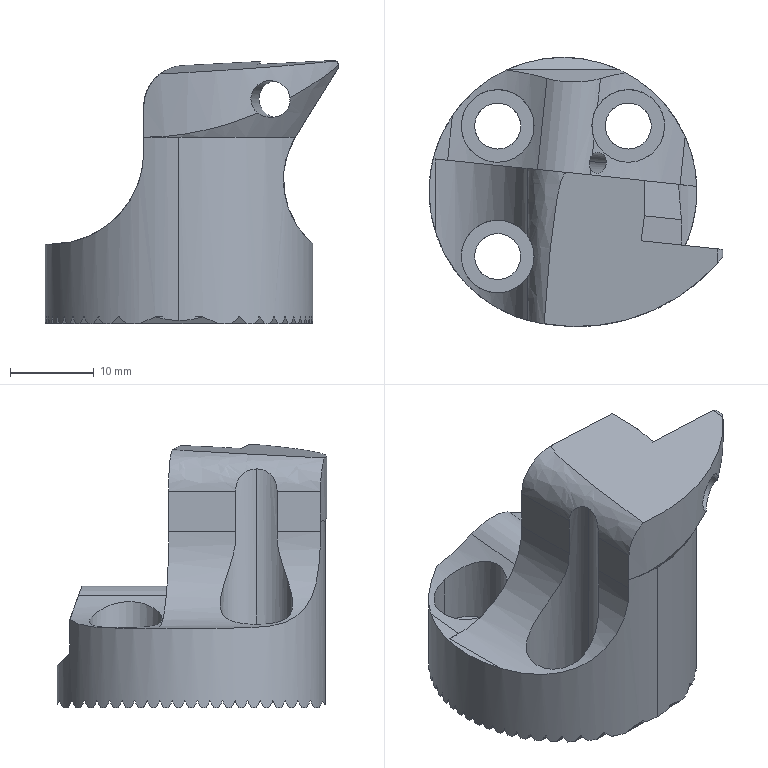NC program | Mastercam | posted with a generic post
Lines 4934 to 6578 of 7170:
(4 FEMR |TOOL - 5|DIA. OFF. - 5|LEN. - 5|TOOL DIA. - 4.)
N9924 T5 M6
N9926 G0 G54 G90 X45.762 Y19.276 C6. B-90. S4000 M3
N9928 G43 H5 Z52.023
N9930 Z3.023
N9932 G1 Z1.825 F2000.
N9934 G41 D5 X44.822 Y18.934 F600.
N9936 X30.436 Y13.698
N9938 X27.418 Y11.34
N9940 X31.243 Y11.54
N9942 X45.536 Y17.027
N9944 G40 X46.469 Y17.385
N9946 X45.078 Y21.156
N9948 G41 D5 X44.138 Y20.814
N9950 X29.455 Y15.469
N9952 X21.188 Y9.01
N9954 X31.664 Y9.56
N9956 X46.252 Y15.159
N9958 G40 X47.186 Y15.518
N9960 X45.762 Y19.276
N9962 Z1.627 F2000.
N9964 G41 D5 X44.822 Y18.934 F600.
N9966 X30.436 Y13.698
N9968 X27.418 Y11.34
N9970 X31.243 Y11.54
N9972 X45.536 Y17.027
N9974 G40 X46.469 Y17.385
N9976 X45.078 Y21.156
N9978 G41 D5 X44.138 Y20.814
N9980 X29.455 Y15.469
N9982 X21.188 Y9.01
N9984 X31.664 Y9.56
N9986 X46.252 Y15.159
N9988 G40 X47.186 Y15.518
N9990 X45.762 Y19.276
N9992 Z1.43 F2000.
N9994 G41 D5 X44.822 Y18.934 F600.
N9996 X30.436 Y13.698
N9998 X27.418 Y11.34
N100 X31.243 Y11.54
N102 X45.536 Y17.027
N104 G40 X46.469 Y17.385
N106 X45.078 Y21.156
N108 G41 D5 X44.138 Y20.814
N110 X29.455 Y15.469
N112 X21.188 Y9.01
N114 X31.664 Y9.56
N116 X46.252 Y15.159
N118 G40 X47.186 Y15.518
N120 X45.762 Y19.276
N122 Z1.232 F2000.
N124 G41 D5 X44.822 Y18.934 F600.
N126 X30.436 Y13.698
N128 X27.418 Y11.34
N130 X31.243 Y11.54
N132 X45.536 Y17.027
N134 G40 X46.469 Y17.385
N136 X45.078 Y21.156
N138 G41 D5 X44.138 Y20.814
N140 X29.455 Y15.469
N142 X21.188 Y9.01
N144 X31.664 Y9.56
N146 X46.252 Y15.159
N148 G40 X47.186 Y15.518
N150 X45.762 Y19.276
N152 Z1.035 F2000.
N154 G41 D5 X44.822 Y18.934 F600.
N156 X30.436 Y13.698
N158 X27.418 Y11.34
N160 X31.243 Y11.54
N162 X45.536 Y17.027
N164 G40 X46.469 Y17.385
N166 X45.078 Y21.156
N168 G41 D5 X44.138 Y20.814
N170 X29.455 Y15.469
N172 X21.188 Y9.01
N174 X31.664 Y9.56
N176 X46.252 Y15.159
N178 G40 X47.186 Y15.518
N180 X45.762 Y19.276
N182 Z.837 F2000.
N184 G41 D5 X44.822 Y18.934 F600.
N186 X30.436 Y13.698
N188 X27.418 Y11.34
N190 X31.243 Y11.54
N192 X45.536 Y17.027
N194 G40 X46.469 Y17.385
N196 X45.078 Y21.156
N198 G41 D5 X44.138 Y20.814
N200 X29.455 Y15.469
N202 X21.188 Y9.01
N204 X31.664 Y9.56
N206 X46.252 Y15.159
N208 G40 X47.186 Y15.518
N210 X45.762 Y19.276
N212 Z.64 F2000.
N214 G41 D5 X44.822 Y18.934 F600.
N216 X30.436 Y13.698
N218 X27.418 Y11.34
N220 X31.243 Y11.54
N222 X45.536 Y17.027
N224 G40 X46.469 Y17.385
N226 X45.078 Y21.156
N228 G41 D5 X44.138 Y20.814
N230 X29.455 Y15.469
N232 X21.188 Y9.01
N234 X31.664 Y9.56
N236 X46.252 Y15.159
N238 G40 X47.186 Y15.518
N240 X45.762 Y19.276
N242 Z.442 F2000.
N244 G41 D5 X44.822 Y18.934 F600.
N246 X30.436 Y13.698
N248 X27.418 Y11.34
N250 X31.243 Y11.54
N252 X45.536 Y17.027
N254 G40 X46.469 Y17.385
N256 X45.078 Y21.156
N258 G41 D5 X44.138 Y20.814
N260 X29.455 Y15.469
N262 X21.188 Y9.01
N264 X31.664 Y9.56
N266 X46.252 Y15.159
N268 G40 X47.186 Y15.518
N270 X45.762 Y19.276
N272 Z.245 F2000.
N274 G41 D5 X44.822 Y18.934 F600.
N276 X30.436 Y13.698
N278 X27.418 Y11.34
N280 X31.243 Y11.54
N282 X45.536 Y17.027
N284 G40 X46.469 Y17.385
N286 X45.078 Y21.156
N288 G41 D5 X44.138 Y20.814
N290 X29.455 Y15.469
N292 X21.188 Y9.01
N294 X31.664 Y9.56
N296 X46.252 Y15.159
N298 G40 X47.186 Y15.518
N300 X45.762 Y19.276
N302 Z.047 F2000.
N304 G41 D5 X44.822 Y18.934 F600.
N306 X30.436 Y13.698
N308 X27.418 Y11.34
N310 X31.243 Y11.54
N312 X45.536 Y17.027
N314 G40 X46.469 Y17.385
N316 X45.078 Y21.156
N318 G41 D5 X44.138 Y20.814
N320 X29.455 Y15.469
N322 X21.188 Y9.01
N324 X31.664 Y9.56
N326 X46.252 Y15.159
N328 G40 X47.186 Y15.518
N330 X45.762 Y19.276
N332 Z-.151 F2000.
N334 G41 D5 X44.822 Y18.934 F600.
N336 X30.436 Y13.698
N338 X27.418 Y11.34
N340 X31.243 Y11.54
N342 X45.536 Y17.027
N344 G40 X46.469 Y17.385
N346 X45.078 Y21.156
N348 G41 D5 X44.138 Y20.814
N350 X29.455 Y15.469
N352 X21.188 Y9.01
N354 X31.664 Y9.56
N356 X46.252 Y15.159
N358 G40 X47.186 Y15.518
N360 X45.762 Y19.276
N362 Z-.348 F2000.
N364 G41 D5 X44.822 Y18.934 F600.
N366 X30.436 Y13.698
N368 X27.418 Y11.34
N370 X31.243 Y11.54
N372 X45.536 Y17.027
N374 G40 X46.469 Y17.385
N376 X45.078 Y21.156
N378 G41 D5 X44.138 Y20.814
N380 X29.455 Y15.469
N382 X21.188 Y9.01
N384 X31.664 Y9.56
N386 X46.252 Y15.159
N388 G40 X47.186 Y15.518
N390 X45.762 Y19.276
N392 Z-.546 F2000.
N394 G41 D5 X44.822 Y18.934 F600.
N396 X30.436 Y13.698
N398 X27.418 Y11.34
N400 X31.243 Y11.54
N402 X45.536 Y17.027
N404 G40 X46.469 Y17.385
N406 X45.078 Y21.156
N408 G41 D5 X44.138 Y20.814
N410 X29.455 Y15.469
N412 X21.188 Y9.01
N414 X31.664 Y9.56
N416 X46.252 Y15.159
N418 G40 X47.186 Y15.518
N420 X45.762 Y19.276
N422 Z-.743 F2000.
N424 G41 D5 X44.822 Y18.934 F600.
N426 X30.436 Y13.698
N428 X27.418 Y11.34
N430 X31.243 Y11.54
N432 X45.536 Y17.027
N434 G40 X46.469 Y17.385
N436 X45.078 Y21.156
N438 G41 D5 X44.138 Y20.814
N440 X29.455 Y15.469
N442 X21.188 Y9.01
N444 X31.664 Y9.56
N446 X46.252 Y15.159
N448 G40 X47.186 Y15.518
N450 X45.762 Y19.276
N452 Z-.941 F2000.
N454 G41 D5 X44.822 Y18.934 F600.
N456 X30.436 Y13.698
N458 X27.418 Y11.34
N460 X31.243 Y11.54
N462 X45.536 Y17.027
N464 G40 X46.469 Y17.385
N466 X45.078 Y21.156
N468 G41 D5 X44.138 Y20.814
N470 X29.455 Y15.469
N472 X21.188 Y9.01
N474 X31.664 Y9.56
N476 X46.252 Y15.159
N478 G40 X47.186 Y15.518
N480 X45.762 Y19.276
N482 Z-1.138 F2000.
N484 G41 D5 X44.822 Y18.934 F600.
N486 X30.436 Y13.698
N488 X27.418 Y11.34
N490 X31.243 Y11.54
N492 X45.536 Y17.027
N494 G40 X46.469 Y17.385
N496 X45.078 Y21.156
N498 G41 D5 X44.138 Y20.814
N500 X29.455 Y15.469
N502 X21.188 Y9.01
N504 X31.664 Y9.56
N506 X46.252 Y15.159
N508 G40 X47.186 Y15.518
N510 X45.762 Y19.276
N512 Z-1.336 F2000.
N514 G41 D5 X44.822 Y18.934 F600.
N516 X30.436 Y13.698
N518 X27.418 Y11.34
N520 X31.243 Y11.54
N522 X45.536 Y17.027
N524 G40 X46.469 Y17.385
N526 X45.078 Y21.156
N528 G41 D5 X44.138 Y20.814
N530 X29.455 Y15.469
N532 X21.188 Y9.01
N534 X31.664 Y9.56
N536 X46.252 Y15.159
N538 G40 X47.186 Y15.518
N540 X45.762 Y19.276
N542 Z-1.534 F2000.
N544 G41 D5 X44.822 Y18.934 F600.
N546 X30.436 Y13.698
N548 X27.418 Y11.34
N550 X31.243 Y11.54
N552 X45.536 Y17.027
N554 G40 X46.469 Y17.385
N556 X45.078 Y21.156
N558 G41 D5 X44.138 Y20.814
N560 X29.455 Y15.469
N562 X21.188 Y9.01
N564 X31.664 Y9.56
N566 X46.252 Y15.159
N568 G40 X47.186 Y15.518
N570 X45.762 Y19.276
N572 Z-1.731 F2000.
N574 G41 D5 X44.822 Y18.934 F600.
N576 X30.436 Y13.698
N578 X27.418 Y11.34
N580 X31.243 Y11.54
N582 X45.536 Y17.027
N584 G40 X46.469 Y17.385
N586 X45.078 Y21.156
N588 G41 D5 X44.138 Y20.814
N590 X29.455 Y15.469
N592 X21.188 Y9.01
N594 X31.664 Y9.56
N596 X46.252 Y15.159
N598 G40 X47.186 Y15.518
N600 X45.762 Y19.276
N602 Z-1.929 F2000.
N604 G41 D5 X44.822 Y18.934 F600.
N606 X30.436 Y13.698
N608 X27.418 Y11.34
N610 X31.243 Y11.54
N612 X45.536 Y17.027
N614 G40 X46.469 Y17.385
N616 X45.078 Y21.156
N618 G41 D5 X44.138 Y20.814
N620 X29.455 Y15.469
N622 X21.188 Y9.01
N624 X31.664 Y9.56
N626 X46.252 Y15.159
N628 G40 X47.186 Y15.518
N630 X45.762 Y19.276
N632 Z-2.126 F2000.
N634 G41 D5 X44.822 Y18.934 F600.
N636 X30.436 Y13.698
N638 X27.418 Y11.34
N640 X31.243 Y11.54
N642 X45.536 Y17.027
N644 G40 X46.469 Y17.385
N646 X45.078 Y21.156
N648 G41 D5 X44.138 Y20.814
N650 X29.455 Y15.469
N652 X21.188 Y9.01
N654 X31.664 Y9.56
N656 X46.252 Y15.159
N658 G40 X47.186 Y15.518
N660 X45.762 Y19.276
N662 Z-2.324 F2000.
N664 G41 D5 X44.822 Y18.934 F600.
N666 X30.436 Y13.698
N668 X27.418 Y11.34
N670 X31.243 Y11.54
N672 X45.536 Y17.027
N674 G40 X46.469 Y17.385
N676 X45.078 Y21.156
N678 G41 D5 X44.138 Y20.814
N680 X29.455 Y15.469
N682 X21.188 Y9.01
N684 X31.664 Y9.56
N686 X46.252 Y15.159
N688 G40 X47.186 Y15.518
N690 X45.762 Y19.276
N692 Z-2.521 F2000.
N694 G41 D5 X44.822 Y18.934 F600.
N696 X30.436 Y13.698
N698 X27.418 Y11.34
N700 X31.243 Y11.54
N702 X45.536 Y17.027
N704 G40 X46.469 Y17.385
N706 X45.078 Y21.156
N708 G41 D5 X44.138 Y20.814
N710 X29.455 Y15.469
N712 X21.188 Y9.01
N714 X31.664 Y9.56
N716 X46.252 Y15.159
N718 G40 X47.186 Y15.518
N720 X45.762 Y19.276
N722 Z-2.719 F2000.
N724 G41 D5 X44.822 Y18.934 F600.
N726 X30.436 Y13.698
N728 X27.418 Y11.34
N730 X31.243 Y11.54
N732 X45.536 Y17.027
N734 G40 X46.469 Y17.385
N736 X45.078 Y21.156
N738 G41 D5 X44.138 Y20.814
N740 X29.455 Y15.469
N742 X21.188 Y9.01
N744 X31.664 Y9.56
N746 X46.252 Y15.159
N748 G40 X47.186 Y15.518
N750 X45.762 Y19.276
N752 Z-2.916 F2000.
N754 G41 D5 X44.822 Y18.934 F600.
N756 X30.436 Y13.698
N758 X27.418 Y11.34
N760 X31.243 Y11.54
N762 X45.536 Y17.027
N764 G40 X46.469 Y17.385
N766 X45.078 Y21.156
N768 G41 D5 X44.138 Y20.814
N770 X29.455 Y15.469
N772 X21.188 Y9.01
N774 X31.664 Y9.56
N776 X46.252 Y15.159
N778 G40 X47.186 Y15.518
N780 X45.762 Y19.276
N782 Z-3.114 F2000.
N784 G41 D5 X44.822 Y18.934 F600.
N786 X30.436 Y13.698
N788 X27.418 Y11.34
N790 X31.243 Y11.54
N792 X45.536 Y17.027
N794 G40 X46.469 Y17.385
N796 X45.078 Y21.156
N798 G41 D5 X44.138 Y20.814
N800 X29.455 Y15.469
N802 X21.188 Y9.01
N804 X31.664 Y9.56
N806 X46.252 Y15.159
N808 G40 X47.186 Y15.518
N810 X45.762 Y19.276
N812 Z-3.312 F2000.
N814 G41 D5 X44.822 Y18.934 F600.
N816 X30.436 Y13.698
N818 X27.418 Y11.34
N820 X31.243 Y11.54
N822 X45.536 Y17.027
N824 G40 X46.469 Y17.385
N826 X45.078 Y21.156
N828 G41 D5 X44.138 Y20.814
N830 X29.455 Y15.469
N832 X21.188 Y9.01
N834 X31.664 Y9.56
N836 X46.252 Y15.159
N838 G40 X47.186 Y15.518
N840 X45.762 Y19.276
N842 Z-3.509 F2000.
N844 G41 D5 X44.822 Y18.934 F600.
N846 X30.436 Y13.698
N848 X27.418 Y11.34
N850 X31.243 Y11.54
N852 X45.536 Y17.027
N854 G40 X46.469 Y17.385
N856 X45.078 Y21.156
N858 G41 D5 X44.138 Y20.814
N860 X29.455 Y15.469
N862 X21.188 Y9.01
N864 X31.664 Y9.56
N866 X46.252 Y15.159
N868 G40 X47.186 Y15.518
N870 X45.762 Y19.276
N872 Z-3.707 F2000.
N874 G41 D5 X44.822 Y18.934 F600.
N876 X30.436 Y13.698
N878 X27.418 Y11.34
N880 X31.243 Y11.54
N882 X45.536 Y17.027
N884 G40 X46.469 Y17.385
N886 X45.078 Y21.156
N888 G41 D5 X44.138 Y20.814
N890 X29.455 Y15.469
N892 X21.188 Y9.01
N894 X31.664 Y9.56
N896 X46.252 Y15.159
N898 G40 X47.186 Y15.518
N900 X45.762 Y19.276
N902 Z-3.904 F2000.
N904 G41 D5 X44.822 Y18.934 F600.
N906 X30.436 Y13.698
N908 X27.418 Y11.34
N910 X31.243 Y11.54
N912 X45.536 Y17.027
N914 G40 X46.469 Y17.385
N916 X45.078 Y21.156
N918 G41 D5 X44.138 Y20.814
N920 X29.455 Y15.469
N922 X21.188 Y9.01
N924 X31.664 Y9.56
N926 X46.252 Y15.159
N928 G40 X47.186 Y15.518
N930 X45.762 Y19.276
N932 Z-4.102 F2000.
N934 G41 D5 X44.822 Y18.934 F600.
N936 X30.436 Y13.698
N938 X27.418 Y11.34
N940 X31.243 Y11.54
N942 X45.536 Y17.027
N944 G40 X46.469 Y17.385
N946 X45.078 Y21.156
N948 G41 D5 X44.138 Y20.814
N950 X29.455 Y15.469
N952 X21.188 Y9.01
N954 X31.664 Y9.56
N956 X46.252 Y15.159
N958 G40 X47.186 Y15.518
N960 X45.762 Y19.276
N962 Z-4.299 F2000.
N964 G41 D5 X44.822 Y18.934 F600.
N966 X30.436 Y13.698
N968 X27.418 Y11.34
N970 X31.243 Y11.54
N972 X45.536 Y17.027
N974 G40 X46.469 Y17.385
N976 X45.078 Y21.156
N978 G41 D5 X44.138 Y20.814
N980 X29.455 Y15.469
N982 X21.188 Y9.01
N984 X31.664 Y9.56
N986 X46.252 Y15.159
N988 G40 X47.186 Y15.518
N990 X45.762 Y19.276
N992 Z-4.497 F2000.
N994 G41 D5 X44.822 Y18.934 F600.
N996 X30.436 Y13.698
N998 X27.418 Y11.34
N1000 X31.243 Y11.54
N1002 X45.536 Y17.027
N1004 G40 X46.469 Y17.385
N1006 X45.078 Y21.156
N1008 G41 D5 X44.138 Y20.814
N1010 X29.455 Y15.469
N1012 X21.188 Y9.01
N1014 X31.664 Y9.56
N1016 X46.252 Y15.159
N1018 G40 X47.186 Y15.518
N1020 X45.762 Y19.276
N1022 Z-4.694 F2000.
N1024 G41 D5 X44.822 Y18.934 F600.
N1026 X30.436 Y13.698
N1028 X27.418 Y11.34
N1030 X31.243 Y11.54
N1032 X45.536 Y17.027
N1034 G40 X46.469 Y17.385
N1036 X45.078 Y21.156
N1038 G41 D5 X44.138 Y20.814
N1040 X29.455 Y15.469
N1042 X21.188 Y9.01
N1044 X31.664 Y9.56
N1046 X46.252 Y15.159
N1048 G40 X47.186 Y15.518
N1050 X45.762 Y19.276
N1052 Z-4.892 F2000.
N1054 G41 D5 X44.822 Y18.934 F600.
N1056 X30.436 Y13.698
N1058 X27.418 Y11.34
N1060 X31.243 Y11.54
N1062 X45.536 Y17.027
N1064 G40 X46.469 Y17.385
N1066 X45.078 Y21.156
N1068 G41 D5 X44.138 Y20.814
N1070 X29.455 Y15.469
N1072 X21.188 Y9.01
N1074 X31.664 Y9.56
N1076 X46.252 Y15.159
N1078 G40 X47.186 Y15.518
N1080 X45.762 Y19.276
N1082 Z-5.09 F2000.
N1084 G41 D5 X44.822 Y18.934 F600.
N1086 X30.436 Y13.698
N1088 X27.418 Y11.34
N1090 X31.243 Y11.54
N1092 X45.536 Y17.027
N1094 G40 X46.469 Y17.385
N1096 X45.078 Y21.156
N1098 G41 D5 X44.138 Y20.814
N1100 X29.455 Y15.469
N1102 X21.188 Y9.01
N1104 X31.664 Y9.56
N1106 X46.252 Y15.159
N1108 G40 X47.186 Y15.518
N1110 X45.762 Y19.276
N1112 Z-5.287 F2000.
N1114 G41 D5 X44.822 Y18.934 F600.
N1116 X30.436 Y13.698
N1118 X27.418 Y11.34
N1120 X31.243 Y11.54
N1122 X45.536 Y17.027
N1124 G40 X46.469 Y17.385
N1126 X45.078 Y21.156
N1128 G41 D5 X44.138 Y20.814
N1130 X29.455 Y15.469
N1132 X21.188 Y9.01
N1134 X31.664 Y9.56
N1136 X46.252 Y15.159
N1138 G40 X47.186 Y15.518
N1140 X45.762 Y19.276
N1142 Z-5.485 F2000.
N1144 G41 D5 X44.822 Y18.934 F600.
N1146 X30.436 Y13.698
N1148 X27.418 Y11.34
N1150 X31.243 Y11.54
N1152 X45.536 Y17.027
N1154 G40 X46.469 Y17.385
N1156 X45.078 Y21.156
N1158 G41 D5 X44.138 Y20.814
N1160 X29.455 Y15.469
N1162 X21.188 Y9.01
N1164 X31.664 Y9.56
N1166 X46.252 Y15.159
N1168 G40 X47.186 Y15.518
N1170 X45.762 Y19.276
N1172 Z-5.682 F2000.
N1174 G41 D5 X44.822 Y18.934 F600.
N1176 X30.436 Y13.698
N1178 X27.418 Y11.34
N1180 X31.243 Y11.54
N1182 X45.536 Y17.027
N1184 G40 X46.469 Y17.385
N1186 X45.078 Y21.156
N1188 G41 D5 X44.138 Y20.814
N1190 X29.455 Y15.469
N1192 X21.188 Y9.01
N1194 X31.664 Y9.56
N1196 X46.252 Y15.159
N1198 G40 X47.186 Y15.518
N1200 X45.762 Y19.276
N1202 Z-5.88 F2000.
N1204 G41 D5 X44.822 Y18.934 F600.
N1206 X30.436 Y13.698
N1208 X27.418 Y11.34
N1210 X31.243 Y11.54
N1212 X45.536 Y17.027
N1214 G40 X46.469 Y17.385
N1216 X45.078 Y21.156
N1218 G41 D5 X44.138 Y20.814
N1220 X29.455 Y15.469
N1222 X21.188 Y9.01
N1224 X31.664 Y9.56
N1226 X46.252 Y15.159
N1228 G40 X47.186 Y15.518
N1230 X45.762 Y19.276
N1232 Z-6.077 F2000.
N1234 G41 D5 X44.822 Y18.934 F600.
N1236 X30.436 Y13.698
N1238 X27.418 Y11.34
N1240 X31.243 Y11.54
N1242 X45.536 Y17.027
N1244 G40 X46.469 Y17.385
N1246 X45.078 Y21.156
N1248 G41 D5 X44.138 Y20.814
N1250 X29.455 Y15.469
N1252 X21.188 Y9.01
N1254 X31.664 Y9.56
N1256 X46.252 Y15.159
N1258 G40 X47.186 Y15.518
N1260 G0 Z52.023
N1262 M5
N1264 G0 G28 G91 Z0.
N1266 G28 C0. B0.
N1268 M01
N1270 G0 G17 G40 G80 G90 G94 G98
N1272 G0 G28 G91 Z0.
(3 FEMR |TOOL - 6|DIA. OFF. - 6|LEN. - 6|TOOL DIA. - 3.)
N1274 T6 M6
N1276 G0 G54 G90 X22.325 Y9.265 C6. B-90. S4500 M3
N1278 G43 H6 Z51.993
N1280 Z2.993
N1282 G1 Z1.796 F2000.
N1284 G41 D6 X22.017 Y9.659 F400.
N1286 G3 X21.623 Y9.851 I-.394 J-.308
N1288 X21.316 Y9.745 J-.5
N1290 G1 X20.155 Y8.838
N1292 X14.158 Y6.596
N1294 G3 X14.027 Y6.408 I.07 J-.188
N1296 X14.228 Y6.207 I.201
N1298 X14.298 Y6.221 J.201
N1300 G1 X20.295 Y8.463
N1302 X21.785 Y8.541
N1304 G3 X22.259 Y9.04 I-.026 J.499
N1306 X22.258 Y9.067 I-.5
N1308 G1 G40 X22.232 Y9.566
N1310 X22.325 Y9.265
N1312 Z1.599 F2000.
N1314 G41 D6 X22.017 Y9.659 F400.
N1316 G3 X21.623 Y9.851 I-.394 J-.308
N1318 X21.316 Y9.745 J-.5
N1320 G1 X20.155 Y8.838
N1322 X14.158 Y6.596
N1324 G3 X14.027 Y6.408 I.07 J-.188
N1326 X14.228 Y6.207 I.201
N1328 X14.298 Y6.221 J.201
N1330 G1 X20.295 Y8.463
N1332 X21.785 Y8.541
N1334 G3 X22.259 Y9.04 I-.026 J.499
N1336 X22.258 Y9.067 I-.5
N1338 G1 G40 X22.232 Y9.566
N1340 X22.325 Y9.265
N1342 Z1.402 F2000.
N1344 G41 D6 X22.017 Y9.659 F400.
N1346 G3 X21.623 Y9.851 I-.394 J-.308
N1348 X21.316 Y9.745 J-.5
N1350 G1 X20.155 Y8.838
N1352 X14.158 Y6.596
N1354 G3 X14.027 Y6.408 I.07 J-.188
N1356 X14.228 Y6.207 I.201
N1358 X14.298 Y6.221 J.201
N1360 G1 X20.295 Y8.463
N1362 X21.785 Y8.541
N1364 G3 X22.259 Y9.04 I-.026 J.499
N1366 X22.258 Y9.067 I-.5
N1368 G1 G40 X22.232 Y9.566
N1370 X22.325 Y9.265
N1372 Z1.205 F2000.
N1374 G41 D6 X22.017 Y9.659 F400.
N1376 G3 X21.623 Y9.851 I-.394 J-.308
N1378 X21.316 Y9.745 J-.5
N1380 G1 X20.155 Y8.838
N1382 X14.158 Y6.596
N1384 G3 X14.027 Y6.408 I.07 J-.188
N1386 X14.228 Y6.207 I.201
N1388 X14.298 Y6.221 J.201
N1390 G1 X20.295 Y8.463
N1392 X21.785 Y8.541
N1394 G3 X22.259 Y9.04 I-.026 J.499
N1396 X22.258 Y9.067 I-.5
N1398 G1 G40 X22.232 Y9.566
N1400 X22.325 Y9.265
N1402 Z1.008 F2000.
N1404 G41 D6 X22.017 Y9.659 F400.
N1406 G3 X21.623 Y9.851 I-.394 J-.308
N1408 X21.316 Y9.745 J-.5
N1410 G1 X20.155 Y8.838
N1412 X14.158 Y6.596
N1414 G3 X14.027 Y6.408 I.07 J-.188
N1416 X14.228 Y6.207 I.201
N1418 X14.298 Y6.221 J.201
N1420 G1 X20.295 Y8.463
N1422 X21.785 Y8.541
N1424 G3 X22.259 Y9.04 I-.026 J.499
N1426 X22.258 Y9.067 I-.5
N1428 G1 G40 X22.232 Y9.566
N1430 X22.325 Y9.265
N1432 Z.812 F2000.
N1434 G41 D6 X22.017 Y9.659 F400.
N1436 G3 X21.623 Y9.851 I-.394 J-.308
N1438 X21.316 Y9.745 J-.5
N1440 G1 X20.155 Y8.838
N1442 X14.158 Y6.596
N1444 G3 X14.027 Y6.408 I.07 J-.188
N1446 X14.228 Y6.207 I.201
N1448 X14.298 Y6.221 J.201
N1450 G1 X20.295 Y8.463
N1452 X21.785 Y8.541
N1454 G3 X22.259 Y9.04 I-.026 J.499
N1456 X22.258 Y9.067 I-.5
N1458 G1 G40 X22.232 Y9.566
N1460 X22.325 Y9.265
N1462 Z.615 F2000.
N1464 G41 D6 X22.017 Y9.659 F400.
N1466 G3 X21.623 Y9.851 I-.394 J-.308
N1468 X21.316 Y9.745 J-.5
N1470 G1 X20.155 Y8.838
N1472 X14.158 Y6.596
N1474 G3 X14.027 Y6.408 I.07 J-.188
N1476 X14.228 Y6.207 I.201
N1478 X14.298 Y6.221 J.201
N1480 G1 X20.295 Y8.463
N1482 X21.785 Y8.541
N1484 G3 X22.259 Y9.04 I-.026 J.499
N1486 X22.258 Y9.067 I-.5
N1488 G1 G40 X22.232 Y9.566
N1490 X22.325 Y9.265
N1492 Z.418 F2000.
N1494 G41 D6 X22.017 Y9.659 F400.
N1496 G3 X21.623 Y9.851 I-.394 J-.308
N1498 X21.316 Y9.745 J-.5
N1500 G1 X20.155 Y8.838
N1502 X14.158 Y6.596
N1504 G3 X14.027 Y6.408 I.07 J-.188
N1506 X14.228 Y6.207 I.201
N1508 X14.298 Y6.221 J.201
N1510 G1 X20.295 Y8.463
N1512 X21.785 Y8.541
N1514 G3 X22.259 Y9.04 I-.026 J.499
N1516 X22.258 Y9.067 I-.5
N1518 G1 G40 X22.232 Y9.566
N1520 X22.325 Y9.265
N1522 Z.221 F2000.
N1524 G41 D6 X22.017 Y9.659 F400.
N1526 G3 X21.623 Y9.851 I-.394 J-.308
N1528 X21.316 Y9.745 J-.5
N1530 G1 X20.155 Y8.838
N1532 X14.158 Y6.596
N1534 G3 X14.027 Y6.408 I.07 J-.188
N1536 X14.228 Y6.207 I.201
N1538 X14.298 Y6.221 J.201
N1540 G1 X20.295 Y8.463
N1542 X21.785 Y8.541
N1544 G3 X22.259 Y9.04 I-.026 J.499
N1546 X22.258 Y9.067 I-.5
N1548 G1 G40 X22.232 Y9.566
N1550 X22.325 Y9.265
N1552 Z.024 F2000.
N1554 G41 D6 X22.017 Y9.659 F400.
N1556 G3 X21.623 Y9.851 I-.394 J-.308
N1558 X21.316 Y9.745 J-.5
N1560 G1 X20.155 Y8.838
N1562 X14.158 Y6.596
N1564 G3 X14.027 Y6.408 I.07 J-.188
N1566 X14.228 Y6.207 I.201
N1568 X14.298 Y6.221 J.201
N1570 G1 X20.295 Y8.463
N1572 X21.785 Y8.541
N1574 G3 X22.259 Y9.04 I-.026 J.499
N1576 X22.258 Y9.067 I-.5
N1578 G1 G40 X22.232 Y9.566
N1580 X22.325 Y9.265
N1582 Z-.173 F2000.
N1584 G41 D6 X22.017 Y9.659 F400.
N1586 G3 X21.623 Y9.851 I-.394 J-.308
N1588 X21.316 Y9.745 J-.5
N1590 G1 X20.155 Y8.838
N1592 X14.158 Y6.596
N1594 G3 X14.027 Y6.408 I.07 J-.188
N1596 X14.228 Y6.207 I.201
N1598 X14.298 Y6.221 J.201
N1600 G1 X20.295 Y8.463
N1602 X21.785 Y8.541
N1604 G3 X22.259 Y9.04 I-.026 J.499
N1606 X22.258 Y9.067 I-.5
N1608 G1 G40 X22.232 Y9.566
N1610 X22.325 Y9.265
N1612 Z-.369 F2000.
N1614 G41 D6 X22.017 Y9.659 F400.
N1616 G3 X21.623 Y9.851 I-.394 J-.308
N1618 X21.316 Y9.745 J-.5
N1620 G1 X20.155 Y8.838
N1622 X14.158 Y6.596
N1624 G3 X14.027 Y6.408 I.07 J-.188
N1626 X14.228 Y6.207 I.201
N1628 X14.298 Y6.221 J.201
N1630 G1 X20.295 Y8.463
N1632 X21.785 Y8.541
N1634 G3 X22.259 Y9.04 I-.026 J.499
N1636 X22.258 Y9.067 I-.5
N1638 G1 G40 X22.232 Y9.566
N1640 X22.325 Y9.265
N1642 Z-.566 F2000.
N1644 G41 D6 X22.017 Y9.659 F400.
N1646 G3 X21.623 Y9.851 I-.394 J-.308
N1648 X21.316 Y9.745 J-.5
N1650 G1 X20.155 Y8.838
N1652 X14.158 Y6.596
N1654 G3 X14.027 Y6.408 I.07 J-.188
N1656 X14.228 Y6.207 I.201
N1658 X14.298 Y6.221 J.201
N1660 G1 X20.295 Y8.463
N1662 X21.785 Y8.541
N1664 G3 X22.259 Y9.04 I-.026 J.499
N1666 X22.258 Y9.067 I-.5
N1668 G1 G40 X22.232 Y9.566
N1670 X22.325 Y9.265
N1672 Z-.763 F2000.
N1674 G41 D6 X22.017 Y9.659 F400.
N1676 G3 X21.623 Y9.851 I-.394 J-.308
N1678 X21.316 Y9.745 J-.5
N1680 G1 X20.155 Y8.838
N1682 X14.158 Y6.596
N1684 G3 X14.027 Y6.408 I.07 J-.188
N1686 X14.228 Y6.207 I.201
N1688 X14.298 Y6.221 J.201
N1690 G1 X20.295 Y8.463
N1692 X21.785 Y8.541
N1694 G3 X22.259 Y9.04 I-.026 J.499
N1696 X22.258 Y9.067 I-.5
N1698 G1 G40 X22.232 Y9.566
N1700 X22.325 Y9.265
N1702 Z-.96 F2000.
N1704 G41 D6 X22.017 Y9.659 F400.
N1706 G3 X21.623 Y9.851 I-.394 J-.308
N1708 X21.316 Y9.745 J-.5
N1710 G1 X20.155 Y8.838
N1712 X14.158 Y6.596
N1714 G3 X14.027 Y6.408 I.07 J-.188
N1716 X14.228 Y6.207 I.201
N1718 X14.298 Y6.221 J.201
N1720 G1 X20.295 Y8.463
N1722 X21.785 Y8.541
N1724 G3 X22.259 Y9.04 I-.026 J.499
N1726 X22.258 Y9.067 I-.5
N1728 G1 G40 X22.232 Y9.566
N1730 X22.325 Y9.265
N1732 Z-1.157 F2000.
N1734 G41 D6 X22.017 Y9.659 F400.
N1736 G3 X21.623 Y9.851 I-.394 J-.308
N1738 X21.316 Y9.745 J-.5
N1740 G1 X20.155 Y8.838
N1742 X14.158 Y6.596
N1744 G3 X14.027 Y6.408 I.07 J-.188
N1746 X14.228 Y6.207 I.201
N1748 X14.298 Y6.221 J.201
N1750 G1 X20.295 Y8.463
N1752 X21.785 Y8.541
N1754 G3 X22.259 Y9.04 I-.026 J.499
N1756 X22.258 Y9.067 I-.5
N1758 G1 G40 X22.232 Y9.566
N1760 X22.325 Y9.265
N1762 Z-1.354 F2000.
N1764 G41 D6 X22.017 Y9.659 F400.
N1766 G3 X21.623 Y9.851 I-.394 J-.308
N1768 X21.316 Y9.745 J-.5
N1770 G1 X20.155 Y8.838
N1772 X14.158 Y6.596
N1774 G3 X14.027 Y6.408 I.07 J-.188
N1776 X14.228 Y6.207 I.201
N1778 X14.298 Y6.221 J.201
N1780 G1 X20.295 Y8.463
N1782 X21.785 Y8.541
N1784 G3 X22.259 Y9.04 I-.026 J.499
N1786 X22.258 Y9.067 I-.5
N1788 G1 G40 X22.232 Y9.566
N1790 X22.325 Y9.265
N1792 Z-1.55 F2000.
N1794 G41 D6 X22.017 Y9.659 F400.
N1796 G3 X21.623 Y9.851 I-.394 J-.308
N1798 X21.316 Y9.745 J-.5
N1800 G1 X20.155 Y8.838
N1802 X14.158 Y6.596
N1804 G3 X14.027 Y6.408 I.07 J-.188
N1806 X14.228 Y6.207 I.201
N1808 X14.298 Y6.221 J.201
N1810 G1 X20.295 Y8.463
N1812 X21.785 Y8.541
N1814 G3 X22.259 Y9.04 I-.026 J.499
N1816 X22.258 Y9.067 I-.5
N1818 G1 G40 X22.232 Y9.566
N1820 X22.325 Y9.265
N1822 Z-1.747 F2000.
N1824 G41 D6 X22.017 Y9.659 F400.
N1826 G3 X21.623 Y9.851 I-.394 J-.308
N1828 X21.316 Y9.745 J-.5
N1830 G1 X20.155 Y8.838
N1832 X14.158 Y6.596
N1834 G3 X14.027 Y6.408 I.07 J-.188
N1836 X14.228 Y6.207 I.201
N1838 X14.298 Y6.221 J.201
N1840 G1 X20.295 Y8.463
N1842 X21.785 Y8.541
N1844 G3 X22.259 Y9.04 I-.026 J.499
N1846 X22.258 Y9.067 I-.5
N1848 G1 G40 X22.232 Y9.566
N1850 X22.325 Y9.265
N1852 Z-1.944 F2000.
N1854 G41 D6 X22.017 Y9.659 F400.
N1856 G3 X21.623 Y9.851 I-.394 J-.308
N1858 X21.316 Y9.745 J-.5
N1860 G1 X20.155 Y8.838
N1862 X14.158 Y6.596
N1864 G3 X14.027 Y6.408 I.07 J-.188
N1866 X14.228 Y6.207 I.201
N1868 X14.298 Y6.221 J.201
N1870 G1 X20.295 Y8.463
N1872 X21.785 Y8.541
N1874 G3 X22.259 Y9.04 I-.026 J.499
N1876 X22.258 Y9.067 I-.5
N1878 G1 G40 X22.232 Y9.566
N1880 X22.325 Y9.265
N1882 Z-2.141 F2000.
N1884 G41 D6 X22.017 Y9.659 F400.
N1886 G3 X21.623 Y9.851 I-.394 J-.308
N1888 X21.316 Y9.745 J-.5
N1890 G1 X20.155 Y8.838
N1892 X14.158 Y6.596
N1894 G3 X14.027 Y6.408 I.07 J-.188
N1896 X14.228 Y6.207 I.201
N1898 X14.298 Y6.221 J.201
N1900 G1 X20.295 Y8.463
N1902 X21.785 Y8.541
N1904 G3 X22.259 Y9.04 I-.026 J.499
N1906 X22.258 Y9.067 I-.5
N1908 G1 G40 X22.232 Y9.566
N1910 X22.325 Y9.265
N1912 Z-2.338 F2000.
N1914 G41 D6 X22.017 Y9.659 F400.
N1916 G3 X21.623 Y9.851 I-.394 J-.308
N1918 X21.316 Y9.745 J-.5
N1920 G1 X20.155 Y8.838
N1922 X14.158 Y6.596
N1924 G3 X14.027 Y6.408 I.07 J-.188
N1926 X14.228 Y6.207 I.201
N1928 X14.298 Y6.221 J.201
N1930 G1 X20.295 Y8.463
N1932 X21.785 Y8.541
N1934 G3 X22.259 Y9.04 I-.026 J.499
N1936 X22.258 Y9.067 I-.5
N1938 G1 G40 X22.232 Y9.566
N1940 X22.325 Y9.265
N1942 Z-2.534 F2000.
N1944 G41 D6 X22.017 Y9.659 F400.
N1946 G3 X21.623 Y9.851 I-.394 J-.308
N1948 X21.316 Y9.745 J-.5
N1950 G1 X20.155 Y8.838
N1952 X14.158 Y6.596
N1954 G3 X14.027 Y6.408 I.07 J-.188
N1956 X14.228 Y6.207 I.201
N1958 X14.298 Y6.221 J.201
N1960 G1 X20.295 Y8.463
N1962 X21.785 Y8.541
N1964 G3 X22.259 Y9.04 I-.026 J.499
N1966 X22.258 Y9.067 I-.5
N1968 G1 G40 X22.232 Y9.566
N1970 X22.325 Y9.265
N1972 Z-2.731 F2000.
N1974 G41 D6 X22.017 Y9.659 F400.
N1976 G3 X21.623 Y9.851 I-.394 J-.308
N1978 X21.316 Y9.745 J-.5
N1980 G1 X20.155 Y8.838
N1982 X14.158 Y6.596
N1984 G3 X14.027 Y6.408 I.07 J-.188
N1986 X14.228 Y6.207 I.201
N1988 X14.298 Y6.221 J.201
N1990 G1 X20.295 Y8.463
N1992 X21.785 Y8.541
N1994 G3 X22.259 Y9.04 I-.026 J.499
N1996 X22.258 Y9.067 I-.5
N1998 G1 G40 X22.232 Y9.566
N2000 X22.325 Y9.265
N2002 Z-2.928 F2000.
N2004 G41 D6 X22.017 Y9.659 F400.
N2006 G3 X21.623 Y9.851 I-.394 J-.308
N2008 X21.316 Y9.745 J-.5
N2010 G1 X20.155 Y8.838
N2012 X14.158 Y6.596
N2014 G3 X14.027 Y6.408 I.07 J-.188
N2016 X14.228 Y6.207 I.201
N2018 X14.298 Y6.221 J.201
N2020 G1 X20.295 Y8.463
N2022 X21.785 Y8.541
N2024 G3 X22.259 Y9.04 I-.026 J.499
N2026 X22.258 Y9.067 I-.5
N2028 G1 G40 X22.232 Y9.566
N2030 X22.325 Y9.265
N2032 Z-3.125 F2000.
N2034 G41 D6 X22.017 Y9.659 F400.
N2036 G3 X21.623 Y9.851 I-.394 J-.308
N2038 X21.316 Y9.745 J-.5
N2040 G1 X20.155 Y8.838
N2042 X14.158 Y6.596
N2044 G3 X14.027 Y6.408 I.07 J-.188
N2046 X14.228 Y6.207 I.201
N2048 X14.298 Y6.221 J.201
N2050 G1 X20.295 Y8.463
N2052 X21.785 Y8.541
N2054 G3 X22.259 Y9.04 I-.026 J.499
N2056 X22.258 Y9.067 I-.5
N2058 G1 G40 X22.232 Y9.566
N2060 X22.325 Y9.265
N2062 Z-3.322 F2000.
N2064 G41 D6 X22.017 Y9.659 F400.
N2066 G3 X21.623 Y9.851 I-.394 J-.308
N2068 X21.316 Y9.745 J-.5
N2070 G1 X20.155 Y8.838
N2072 X14.158 Y6.596
N2074 G3 X14.027 Y6.408 I.07 J-.188
N2076 X14.228 Y6.207 I.201
N2078 X14.298 Y6.221 J.201
N2080 G1 X20.295 Y8.463
N2082 X21.785 Y8.541
N2084 G3 X22.259 Y9.04 I-.026 J.499
N2086 X22.258 Y9.067 I-.5
N2088 G1 G40 X22.232 Y9.566
N2090 X22.325 Y9.265
N2092 Z-3.519 F2000.
N2094 G41 D6 X22.017 Y9.659 F400.
N2096 G3 X21.623 Y9.851 I-.394 J-.308
N2098 X21.316 Y9.745 J-.5
N2100 G1 X20.155 Y8.838
N2102 X14.158 Y6.596
N2104 G3 X14.027 Y6.408 I.07 J-.188
N2106 X14.228 Y6.207 I.201
N2108 X14.298 Y6.221 J.201
N2110 G1 X20.295 Y8.463
N2112 X21.785 Y8.541
N2114 G3 X22.259 Y9.04 I-.026 J.499
N2116 X22.258 Y9.067 I-.5
N2118 G1 G40 X22.232 Y9.566
N2120 X22.325 Y9.265
N2122 Z-3.715 F2000.
N2124 G41 D6 X22.017 Y9.659 F400.
N2126 G3 X21.623 Y9.851 I-.394 J-.308
N2128 X21.316 Y9.745 J-.5
N2130 G1 X20.155 Y8.838
N2132 X14.158 Y6.596
N2134 G3 X14.027 Y6.408 I.07 J-.188
N2136 X14.228 Y6.207 I.201
N2138 X14.298 Y6.221 J.201
N2140 G1 X20.295 Y8.463
N2142 X21.785 Y8.541
N2144 G3 X22.259 Y9.04 I-.026 J.499
N2146 X22.258 Y9.067 I-.5
N2148 G1 G40 X22.232 Y9.566
N2150 X22.325 Y9.265
N2152 Z-3.912 F2000.
N2154 G41 D6 X22.017 Y9.659 F400.
N2156 G3 X21.623 Y9.851 I-.394 J-.308
N2158 X21.316 Y9.745 J-.5
N2160 G1 X20.155 Y8.838
N2162 X14.158 Y6.596
N2164 G3 X14.027 Y6.408 I.07 J-.188
N2166 X14.228 Y6.207 I.201
N2168 X14.298 Y6.221 J.201
N2170 G1 X20.295 Y8.463
N2172 X21.785 Y8.541
N2174 G3 X22.259 Y9.04 I-.026 J.499
N2176 X22.258 Y9.067 I-.5
N2178 G1 G40 X22.232 Y9.566
N2180 X22.325 Y9.265
N2182 Z-4.109 F2000.
N2184 G41 D6 X22.017 Y9.659 F400.
N2186 G3 X21.623 Y9.851 I-.394 J-.308
N2188 X21.316 Y9.745 J-.5
N2190 G1 X20.155 Y8.838
N2192 X14.158 Y6.596
N2194 G3 X14.027 Y6.408 I.07 J-.188
N2196 X14.228 Y6.207 I.201
N2198 X14.298 Y6.221 J.201
N2200 G1 X20.295 Y8.463
N2202 X21.785 Y8.541
N2204 G3 X22.259 Y9.04 I-.026 J.499
N2206 X22.258 Y9.067 I-.5
N2208 G1 G40 X22.232 Y9.566
N2210 X22.325 Y9.265
N2212 Z-4.306 F2000.
N2214 G41 D6 X22.017 Y9.659 F400.
N2216 G3 X21.623 Y9.851 I-.394 J-.308
N2218 X21.316 Y9.745 J-.5
N2220 G1 X20.155 Y8.838
N2222 X14.158 Y6.596
N2224 G3 X14.027 Y6.408 I.07 J-.188
N2226 X14.228 Y6.207 I.201
N2228 X14.298 Y6.221 J.201
N2230 G1 X20.295 Y8.463
N2232 X21.785 Y8.541
N2234 G3 X22.259 Y9.04 I-.026 J.499
N2236 X22.258 Y9.067 I-.5
N2238 G1 G40 X22.232 Y9.566
N2240 X22.325 Y9.265
N2242 Z-4.503 F2000.
N2244 G41 D6 X22.017 Y9.659 F400.
N2246 G3 X21.623 Y9.851 I-.394 J-.308
N2248 X21.316 Y9.745 J-.5
N2250 G1 X20.155 Y8.838
N2252 X14.158 Y6.596
N2254 G3 X14.027 Y6.408 I.07 J-.188
N2256 X14.228 Y6.207 I.201
N2258 X14.298 Y6.221 J.201
N2260 G1 X20.295 Y8.463
N2262 X21.785 Y8.541
N2264 G3 X22.259 Y9.04 I-.026 J.499
N2266 X22.258 Y9.067 I-.5
N2268 G1 G40 X22.232 Y9.566
N2270 X22.325 Y9.265
N2272 Z-4.7 F2000.
N2274 G41 D6 X22.017 Y9.659 F400.
N2276 G3 X21.623 Y9.851 I-.394 J-.308
N2278 X21.316 Y9.745 J-.5
N2280 G1 X20.155 Y8.838
N2282 X14.158 Y6.596
N2284 G3 X14.027 Y6.408 I.07 J-.188
N2286 X14.228 Y6.207 I.201
N2288 X14.298 Y6.221 J.201
N2290 G1 X20.295 Y8.463
N2292 X21.785 Y8.541
N2294 G3 X22.259 Y9.04 I-.026 J.499
N2296 X22.258 Y9.067 I-.5
N2298 G1 G40 X22.232 Y9.566
N2300 X22.325 Y9.265
N2302 Z-4.896 F2000.
N2304 G41 D6 X22.017 Y9.659 F400.
N2306 G3 X21.623 Y9.851 I-.394 J-.308
N2308 X21.316 Y9.745 J-.5
N2310 G1 X20.155 Y8.838
N2312 X14.158 Y6.596
N2314 G3 X14.027 Y6.408 I.07 J-.188
N2316 X14.228 Y6.207 I.201
N2318 X14.298 Y6.221 J.201
N2320 G1 X20.295 Y8.463
N2322 X21.785 Y8.541
N2324 G3 X22.259 Y9.04 I-.026 J.499
N2326 X22.258 Y9.067 I-.5
N2328 G1 G40 X22.232 Y9.566
N2330 X22.325 Y9.265
N2332 Z-5.093 F2000.
N2334 G41 D6 X22.017 Y9.659 F400.
N2336 G3 X21.623 Y9.851 I-.394 J-.308
N2338 X21.316 Y9.745 J-.5
N2340 G1 X20.155 Y8.838
N2342 X14.158 Y6.596
N2344 G3 X14.027 Y6.408 I.07 J-.188
N2346 X14.228 Y6.207 I.201
N2348 X14.298 Y6.221 J.201
N2350 G1 X20.295 Y8.463
N2352 X21.785 Y8.541
N2354 G3 X22.259 Y9.04 I-.026 J.499
N2356 X22.258 Y9.067 I-.5
N2358 G1 G40 X22.232 Y9.566
N2360 X22.325 Y9.265
N2362 Z-5.29 F2000.
N2364 G41 D6 X22.017 Y9.659 F400.
N2366 G3 X21.623 Y9.851 I-.394 J-.308
N2368 X21.316 Y9.745 J-.5
N2370 G1 X20.155 Y8.838
N2372 X14.158 Y6.596
N2374 G3 X14.027 Y6.408 I.07 J-.188
N2376 X14.228 Y6.207 I.201
N2378 X14.298 Y6.221 J.201
N2380 G1 X20.295 Y8.463
N2382 X21.785 Y8.541
N2384 G3 X22.259 Y9.04 I-.026 J.499
N2386 X22.258 Y9.067 I-.5
N2388 G1 G40 X22.232 Y9.566
N2390 X22.325 Y9.265
N2392 Z-5.487 F2000.
N2394 G41 D6 X22.017 Y9.659 F400.
N2396 G3 X21.623 Y9.851 I-.394 J-.308
N2398 X21.316 Y9.745 J-.5
N2400 G1 X20.155 Y8.838
N2402 X14.158 Y6.596
N2404 G3 X14.027 Y6.408 I.07 J-.188
N2406 X14.228 Y6.207 I.201
N2408 X14.298 Y6.221 J.201
N2410 G1 X20.295 Y8.463
N2412 X21.785 Y8.541
N2414 G3 X22.259 Y9.04 I-.026 J.499
N2416 X22.258 Y9.067 I-.5
N2418 G1 G40 X22.232 Y9.566
N2420 X22.325 Y9.265
N2422 Z-5.684 F2000.
N2424 G41 D6 X22.017 Y9.659 F400.
N2426 G3 X21.623 Y9.851 I-.394 J-.308
N2428 X21.316 Y9.745 J-.5
N2430 G1 X20.155 Y8.838
N2432 X14.158 Y6.596
N2434 G3 X14.027 Y6.408 I.07 J-.188
N2436 X14.228 Y6.207 I.201
N2438 X14.298 Y6.221 J.201
N2440 G1 X20.295 Y8.463
N2442 X21.785 Y8.541
N2444 G3 X22.259 Y9.04 I-.026 J.499
N2446 X22.258 Y9.067 I-.5
N2448 G1 G40 X22.232 Y9.566
N2450 X22.325 Y9.265
N2452 Z-5.881 F2000.
N2454 G41 D6 X22.017 Y9.659 F400.
N2456 G3 X21.623 Y9.851 I-.394 J-.308
N2458 X21.316 Y9.745 J-.5
N2460 G1 X20.155 Y8.838
N2462 X14.158 Y6.596
N2464 G3 X14.027 Y6.408 I.07 J-.188
N2466 X14.228 Y6.207 I.201
N2468 X14.298 Y6.221 J.201
N2470 G1 X20.295 Y8.463
N2472 X21.785 Y8.541
N2474 G3 X22.259 Y9.04 I-.026 J.499
N2476 X22.258 Y9.067 I-.5
N2478 G1 G40 X22.232 Y9.566
N2480 X22.325 Y9.265
N2482 Z-6.077 F2000.
N2484 G41 D6 X22.017 Y9.659 F400.
N2486 G3 X21.623 Y9.851 I-.394 J-.308
N2488 X21.316 Y9.745 J-.5
N2490 G1 X20.155 Y8.838
N2492 X14.158 Y6.596
N2494 G3 X14.027 Y6.408 I.07 J-.188
N2496 X14.228 Y6.207 I.201
N2498 X14.298 Y6.221 J.201
N2500 G1 X20.295 Y8.463
N2502 X21.785 Y8.541
N2504 G3 X22.259 Y9.04 I-.026 J.499
N2506 X22.258 Y9.067 I-.5
N2508 G1 G40 X22.232 Y9.566
N2510 G0 Z51.993
N2512 M5
N2514 G0 G28 G91 Z0.
N2516 G28 C0. B0.
N2518 M01
N2520 G0 G17 G40 G80 G90 G94 G98
N2522 G0 G28 G91 Z0.
(3 FEMF |TOOL - 7|DIA. OFF. - 7|LEN. - 7|TOOL DIA. - 3.)
N2524 T7 M6
N2526 G0 G54 G90 X45.446 Y18.682 C6. B-90. S4500 M3
N2528 G43 H7 Z51.522
N2530 Z2.522
N2532 G1 Z-6.167 F2000.
N2534 G41 D7 X44.976 Y18.511 F400.
N2536 X30.657 Y13.3
N2538 X28.819 Y11.864
N2540 X31.148 Y11.986
N2542 X45.374 Y17.447
N2544 G40 X45.841 Y17.626
N2546 X44.933 Y20.092
N2548 G41 D7 X44.463 Y19.921
N2550 X29.921 Y14.628
N2552 X24.147 Y10.117
N2554 X31.464 Y10.5
N2556 X45.912 Y16.046
N2558 G40 X46.379 Y16.226
N2560 X44.42 Y21.501
N2562 G41 D7 X43.95 Y21.33
N2564 X29.185 Y15.956
N2566 X20.13 Y8.882
N2568 X14.14 Y6.642
N2570 G3 X13.978 Y6.408 I.088 J-.234
N2572 X14.228 Y6.158 I.25
N2574 X14.315 Y6.174 J.25
N2576 G1 X20.305 Y8.413
N2578 X31.78 Y9.015
N2580 X46.45 Y14.646
N2582 G40 X46.916 Y14.825
N2584 G0 Z51.522
N2586 X45.446 Y18.682
N2588 Z2.522
N2590 G1 Z-6.177 F2000.
N2592 G41 D7 X44.976 Y18.511 F400.
N2594 X30.657 Y13.3
N2596 X28.819 Y11.864
N2598 X31.148 Y11.986
N2600 X45.374 Y17.447
N2602 G40 X45.841 Y17.626
N2604 X44.933 Y20.092
N2606 G41 D7 X44.463 Y19.921
N2608 X29.921 Y14.628
N2610 X24.147 Y10.117
N2612 X31.464 Y10.5
N2614 X45.912 Y16.046
N2616 G40 X46.379 Y16.226
N2618 X44.42 Y21.501
N2620 G41 D7 X43.95 Y21.33
N2622 X29.185 Y15.956
N2624 X20.13 Y8.882
N2626 X14.14 Y6.642
N2628 G3 X13.978 Y6.408 I.088 J-.234
N2630 X14.228 Y6.158 I.25
N2632 X14.315 Y6.174 J.25
N2634 G1 X20.305 Y8.413
N2636 X31.78 Y9.015
N2638 X46.45 Y14.646
N2640 G40 X46.916 Y14.825
N2642 G0 Z51.522
N2644 M5
N2646 G0 G28 G91 Z0.
N2648 G28 C0. B0.
N2650 M01
N2652 G0 G17 G40 G80 G90 G94 G98
N2654 G0 G28 G91 Z0.
(2 X 7 DCHC |TOOL - 8|DIA. OFF. - 8|LEN. - 8|TOOL DIA. - 6.)
N2656 T8 M6
N2658 G0 G54 G90 X29.727 Y16.32 C6. B-90. S4000 M3
N2660 G43 H8 Z47.033
N2662 Z-1.967
N2664 G1 Z-4.167 F2000.
N2666 G41 D8 X26.575 Y13.857 F400.
N2668 X19.622 Y8.425
N2670 X29.268 Y8.931
N2672 G40 X33.263 Y9.14
N2674 X29.604 Y16.477
N2676 G41 D8 X26.452 Y14.015
N2678 X18.999 Y8.192
N2680 X29.279 Y8.731
N2682 G40 X33.273 Y8.94
N2684 X29.481 Y16.635
N2686 G41 D8 X26.329 Y14.172
N2688 X18.376 Y7.959
N2690 X29.289 Y8.531
N2692 G40 X33.284 Y8.741
N2694 X29.481 Y16.635
N2696 G41 D8 X26.329 Y14.172
N2698 X18.376 Y7.959
N2700 X29.289 Y8.531
N2702 G40 X33.284 Y8.741
N2704 G0 Z47.033
N2706 M5
N2708 G0 G28 G91 Z0.
N2710 G28 C0. B0.
N2712 M01
N2714 G0 G17 G40 G80 G90 G94 G98
N2716 G0 G28 G91 Z0.
(12 FEMF |TOOL - 9|DIA. OFF. - 9|LEN. - 9|TOOL DIA. - 12.)
N2718 T9 M6
N2720 G0 G54 G90 X15.5 Y24. C6. B-90. S3500 M3
N2722 G43 H9 Z52.593
N2724 Z3.593
N2726 G1 Z2.593 F2000.
N2728 G41 D9 Y16. F600.
N2730 Y-16.
N2732 G40 Y-24.
N2734 G0 Z52.593
N2736 Z64.5
N2738 X12.45 Y14.764
N2740 C0.
N2742 Z15.5
N2744 G1 Z14.5 F2000.
N2746 G41 D9 Y6.764 F600.
N2748 Y-6.764
N2750 G40 Y-14.764
N2752 G0 Z64.5
N2754 X25.185 Y24.045
N2756 Z50.
N2758 Z1.
N2760 G1 Z-12. F2000.
N2762 G41 D9 X25.661 Y21.083 F600.
N2764 G3 X26.154 Y20.663 I.493 J.079
N2766 X26.225 Y20.667 J.499
N2768 G1 X38.825 Y21.324
N2770 G2 X39.153 Y21.333 I.328 J-6.292
N2772 X45.454 Y15.032 J-6.301
N2774 X43.019 Y10.057 I-6.301
N2776 G3 X42.98 Y9.978 I.061 J-.079
N2778 X43.001 Y9.917 I.1
N2780 G1 G40 X44.842 Y7.548
N2782 G0 Z38.
N2784 X25.185 Y24.045
N2786 Z1.
N2788 G1 Z-12. F2000.
N2790 G41 D9 X25.661 Y21.083 F600.
N2792 G3 X26.154 Y20.663 I.493 J.079
N2794 X26.225 Y20.667 J.499
N2796 G1 X38.825 Y21.324
N2798 G2 X39.153 Y21.333 I.328 J-6.292
N2800 X45.454 Y15.032 J-6.301
N2802 X43.019 Y10.057 I-6.301
N2804 G3 X42.98 Y9.978 I.061 J-.079
N2806 X43.001 Y9.917 I.1
N2808 G1 G40 X44.842 Y7.548
N2810 G0 Z50.
N2812 B-270.
N2814 X-15.5 Y-22.5
N2816 Z44.
N2818 Z-5.
N2820 G1 Z-6. F2000.
N2822 G41 D9 Y-16.5 F600.
N2824 Y-12.303
N2826 G3 X-16.273 Y-10.724 I-2.
N2828 G1 X-44.759 Y11.41
N2830 G40 X-49.497 Y15.091
N2832 G0 Z44.
N2834 Z64.849
N2836 X-11.607 Y-14.764
N2838 B-405.
N2840 Z15.849
N2842 G1 Z14.849 F2000.
N2844 G41 D9 Y-6.764 F600.
N2846 Y6.764
N2848 G40 Y14.764
N2850 G0 Z64.849
N2852 M5
N2854 G0 G28 G91 Z0.
N2856 G28 B0.
N2858 M01
N2860 G0 G17 G40 G80 G90 G94 G98
N2862 G0 G28 G91 Z0.
(30 BNOS |TOOL - 10|DIA. OFF. - 10|LEN. - 10|TOOL DIA. - 30.)
N2864 T10 M6
N2866 G0 G54 G90 X24.5 Y31. C6. B-90. S3500 M3
N2868 G43 H10 Z51.793
N2870 Z2.793
N2872 G1 Z1.793 F2000.
N2874 G41 D10 Y16. F600.
N2876 Y-16.
N2878 G40 Y-31.
N2880 G0 Z51.793
N2882 M5
N2884 G0 G28 G91 Z0.
N2886 G28 C0. B0.
N2888 M01
N2890 G0 G17 G40 G80 G90 G94 G98
N2892 G0 G28 G91 Z0.
(6 CHM |TOOL - 12|DIA. OFF. - 12|LEN. - 12|TOOL DIA. - 6.)
N2894 T12 M6
N2896 G0 G54 G90 X27.782 Y11.396 C6. B-90. S2000 M3
N2898 G43 H12 Z43.823
N2900 G81 G98 Z-8.377 R-5.177 F100.
N2902 G80
N2904 M5
N2906 G0 G28 G91 Z0.
N2908 G28 C0. B0.
N2910 M01
N2912 G0 G17 G40 G80 G90 G94 G98
N2914 G0 G28 G91 Z0.
(4.5 DR |TOOL - 13|DIA. OFF. - 13|LEN. - 13|TOOL DIA. - 4.5)
N2916 T13 M6
N2918 G0 G54 G90 X27.782 Y11.396 C6. B-90. S1000 M3
N2920 G43 H13 Z43.823
N2922 G83 G98 Z-16.177 R-5.177 Q2. F60.
N2924 G80
N2926 M5
N2928 G0 G28 G91 Z0.
N2930 G28 C0. B0.
N2932 M01
N2934 G0 G17 G40 G80 G90 G94 G98
N2936 G0 G28 G91 Z0.
(5.5 FEM |TOOL - 11|DIA. OFF. - 11|LEN. - 11|TOOL DIA. - 5.5)
N2938 T11 M6
N2940 G0 G54 G90 X27.782 Y-11.396 C186. B-90. S2500 M3
N2942 G43 H11 Z63.589
N2944 G81 G98 Z10.189 R14.589 F100.
N2946 G80
N2948 M5
N2950 G0 G28 G91 Z0.
N2952 G28 C0. B0.
N2954 M01
N2956 G0 G17 G40 G80 G90 G94 G98
N2958 G0 G28 G91 Z0.
(2.4 THML |TOOL - 14|DIA. OFF. - 14|LEN. - 14|TOOL DIA. - 2.4)
N2960 T14 M6
N2962 G0 G54 G90 X27.782 Y11.396 C6. B-90. S3000 M3
N2964 G43 H14 Z43.823
N2966 Z-4.177
N2968 G1 Z-11.177 F2000.
N2970 G41 D14 X28.887 F300.
N2972 G3 X27.782 Y12.501 Z-11.052 I-1.105
N2974 X26.677 Y11.396 Z-10.927 J-1.105
N2976 X27.782 Y10.291 Z-10.802 I1.105
N2978 X28.887 Y11.396 Z-10.677 J1.105
N2980 X27.782 Y12.501 Z-10.552 I-1.105
N2982 X26.677 Y11.396 Z-10.427 J-1.105
N2984 G1 G40 X27.782
N2986 Z-9.677 F2000.
N2988 G41 D14 X28.887 F300.
N2990 G3 X27.782 Y12.501 Z-9.552 I-1.105
N2992 X26.677 Y11.396 Z-9.427 J-1.105
N2994 X27.782 Y10.291 Z-9.302 I1.105
N2996 X28.887 Y11.396 Z-9.177 J1.105
N2998 X27.782 Y12.501 Z-9.052 I-1.105
N3000 X26.677 Y11.396 Z-8.927 J-1.105
N3002 G1 G40 X27.782
N3004 Z-8.177 F2000.
N3006 G41 D14 X28.887 F300.
N3008 G3 X27.782 Y12.501 Z-8.052 I-1.105
N3010 X26.677 Y11.396 Z-7.927 J-1.105
N3012 X27.782 Y10.291 Z-7.802 I1.105
N3014 X28.887 Y11.396 Z-7.677 J1.105
N3016 X27.782 Y12.501 Z-7.552 I-1.105
N3018 X26.677 Y11.396 Z-7.427 J-1.105
N3020 X27.782 Y10.291 Z-7.302 I1.105
N3022 X28.887 Y11.396 Z-7.177 J1.105
N3024 X27.782 Y12.501 Z-7.052 I-1.105
N3026 X26.677 Y11.396 Z-6.927 J-1.105
N3028 G1 G40 X27.782
N3030 Z-11.177 F2000.
N3032 G41 D14 X28.952 F300.
N3034 G3 X27.782 Y12.566 Z-11.052 I-1.17
N3036 X26.612 Y11.396 Z-10.927 J-1.17
N3038 X27.782 Y10.226 Z-10.802 I1.17
N3040 X28.952 Y11.396 Z-10.677 J1.17
N3042 X27.782 Y12.566 Z-10.552 I-1.17
N3044 X26.612 Y11.396 Z-10.427 J-1.17
N3046 G1 G40 X27.782
N3048 Z-9.677 F2000.
N3050 G41 D14 X28.952 F300.
N3052 G3 X27.782 Y12.566 Z-9.552 I-1.17
N3054 X26.612 Y11.396 Z-9.427 J-1.17
N3056 X27.782 Y10.226 Z-9.302 I1.17
N3058 X28.952 Y11.396 Z-9.177 J1.17
N3060 X27.782 Y12.566 Z-9.052 I-1.17
N3062 X26.612 Y11.396 Z-8.927 J-1.17
N3064 G1 G40 X27.782
N3066 Z-8.177 F2000.
N3068 G41 D14 X28.952 F300.
N3070 G3 X27.782 Y12.566 Z-8.052 I-1.17
N3072 X26.612 Y11.396 Z-7.927 J-1.17
N3074 X27.782 Y10.226 Z-7.802 I1.17
N3076 X28.952 Y11.396 Z-7.677 J1.17
N3078 X27.782 Y12.566 Z-7.552 I-1.17
N3080 X26.612 Y11.396 Z-7.427 J-1.17
N3082 X27.782 Y10.226 Z-7.302 I1.17
N3084 X28.952 Y11.396 Z-7.177 J1.17
N3086 X27.782 Y12.566 Z-7.052 I-1.17
N3088 X26.612 Y11.396 Z-6.927 J-1.17
N3090 G1 G40 X27.782
N3092 Z-11.177 F2000.
N3094 G41 D14 X29.017 F300.
N3096 G3 X27.782 Y12.631 Z-11.052 I-1.235
N3098 X26.547 Y11.396 Z-10.927 J-1.235
N3100 X27.782 Y10.161 Z-10.802 I1.235
N3102 X29.017 Y11.396 Z-10.677 J1.235
N3104 X27.782 Y12.631 Z-10.552 I-1.235
N3106 X26.547 Y11.396 Z-10.427 J-1.235
N3108 G1 G40 X27.782
N3110 Z-9.677 F2000.
N3112 G41 D14 X29.017 F300.
N3114 G3 X27.782 Y12.631 Z-9.552 I-1.235
N3116 X26.547 Y11.396 Z-9.427 J-1.235
N3118 X27.782 Y10.161 Z-9.302 I1.235
N3120 X29.017 Y11.396 Z-9.177 J1.235
N3122 X27.782 Y12.631 Z-9.052 I-1.235
N3124 X26.547 Y11.396 Z-8.927 J-1.235
N3126 G1 G40 X27.782
N3128 Z-8.177 F2000.
N3130 G41 D14 X29.017 F300.
N3132 G3 X27.782 Y12.631 Z-8.052 I-1.235
N3134 X26.547 Y11.396 Z-7.927 J-1.235
N3136 X27.782 Y10.161 Z-7.802 I1.235
N3138 X29.017 Y11.396 Z-7.677 J1.235
N3140 X27.782 Y12.631 Z-7.552 I-1.235
N3142 X26.547 Y11.396 Z-7.427 J-1.235
N3144 X27.782 Y10.161 Z-7.302 I1.235
N3146 X29.017 Y11.396 Z-7.177 J1.235
N3148 X27.782 Y12.631 Z-7.052 I-1.235
N3150 X26.547 Y11.396 Z-6.927 J-1.235
N3152 G1 G40 X27.782
N3154 Z-11.177 F2000.
N3156 G41 D14 X29.082 F300.
N3158 G3 X27.782 Y12.696 Z-11.052 I-1.3
N3160 X26.482 Y11.396 Z-10.927 J-1.3
N3162 X27.782 Y10.096 Z-10.802 I1.3
N3164 X29.082 Y11.396 Z-10.677 J1.3
N3166 X27.782 Y12.696 Z-10.552 I-1.3
N3168 X26.482 Y11.396 Z-10.427 J-1.3
N3170 G1 G40 X27.782
N3172 Z-9.677 F2000.
N3174 G41 D14 X29.082 F300.
N3176 G3 X27.782 Y12.696 Z-9.552 I-1.3
N3178 X26.482 Y11.396 Z-9.427 J-1.3
N3180 X27.782 Y10.096 Z-9.302 I1.3
N3182 X29.082 Y11.396 Z-9.177 J1.3
N3184 X27.782 Y12.696 Z-9.052 I-1.3
N3186 X26.482 Y11.396 Z-8.927 J-1.3
N3188 G1 G40 X27.782
N3190 Z-8.177 F2000.
N3192 G41 D14 X29.082 F300.
N3194 G3 X27.782 Y12.696 Z-8.052 I-1.3
N3196 X26.482 Y11.396 Z-7.927 J-1.3
N3198 X27.782 Y10.096 Z-7.802 I1.3
N3200 X29.082 Y11.396 Z-7.677 J1.3
N3202 X27.782 Y12.696 Z-7.552 I-1.3
N3204 X26.482 Y11.396 Z-7.427 J-1.3
N3206 X27.782 Y10.096 Z-7.302 I1.3
N3208 X29.082 Y11.396 Z-7.177 J1.3
N3210 X27.782 Y12.696 Z-7.052 I-1.3
N3212 X26.482 Y11.396 Z-6.927 J-1.3
N3214 G1 G40 X27.782
N3216 Z-11.177 F2000.
N3218 G41 D14 X29.082 F300.
N3220 G3 X27.782 Y12.696 Z-11.052 I-1.3
N3222 X26.482 Y11.396 Z-10.927 J-1.3
N3224 X27.782 Y10.096 Z-10.802 I1.3
N3226 X29.082 Y11.396 Z-10.677 J1.3
N3228 X27.782 Y12.696 Z-10.552 I-1.3
N3230 X26.482 Y11.396 Z-10.427 J-1.3
N3232 G1 G40 X27.782
N3234 Z-9.677 F2000.
N3236 G41 D14 X29.082 F300.
N3238 G3 X27.782 Y12.696 Z-9.552 I-1.3
N3240 X26.482 Y11.396 Z-9.427 J-1.3
N3242 X27.782 Y10.096 Z-9.302 I1.3
N3244 X29.082 Y11.396 Z-9.177 J1.3
N3246 X27.782 Y12.696 Z-9.052 I-1.3
N3248 X26.482 Y11.396 Z-8.927 J-1.3
N3250 G1 G40 X27.782
N3252 Z-8.177 F2000.
N3254 G41 D14 X29.082 F300.
N3256 G3 X27.782 Y12.696 Z-8.052 I-1.3
N3258 X26.482 Y11.396 Z-7.927 J-1.3
N3260 X27.782 Y10.096 Z-7.802 I1.3
N3262 X29.082 Y11.396 Z-7.677 J1.3
N3264 X27.782 Y12.696 Z-7.552 I-1.3
N3266 X26.482 Y11.396 Z-7.427 J-1.3
N3268 X27.782 Y10.096 Z-7.302 I1.3
N3270 X29.082 Y11.396 Z-7.177 J1.3
N3272 X27.782 Y12.696 Z-7.052 I-1.3
N3274 X26.482 Y11.396 Z-6.927 J-1.3
N3276 G1 G40 X27.782
N3278 G0 Z-4.177
N3280 Z43.823
N3282 M5
N3284 G0 G28 G91 Z0.
N3286 G28 C0. B0.
N3288 M01
N3290 G0 G17 G40 G80 G90 G94 G98
N3292 G0 G28 G91 Z0.